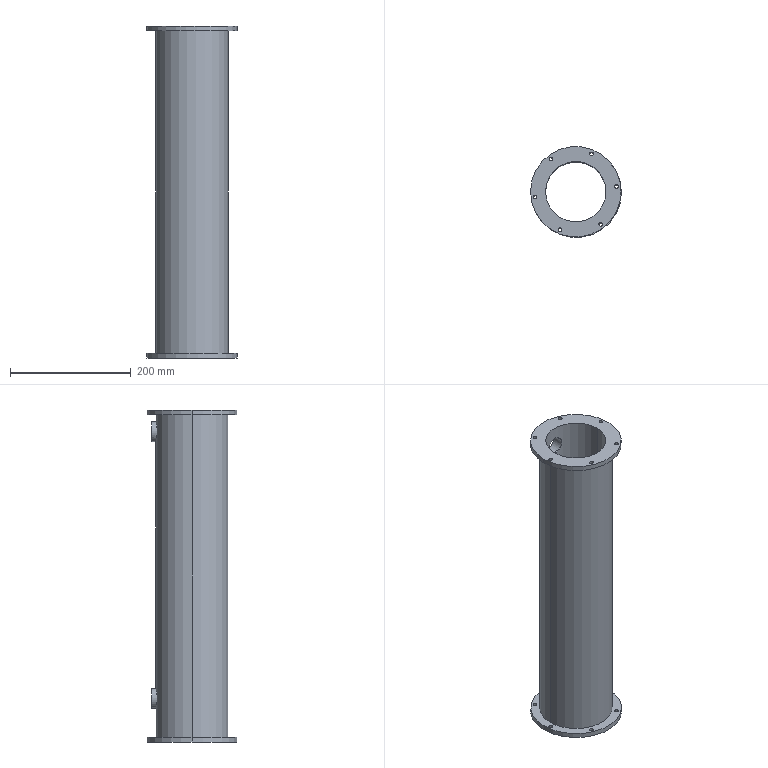Part | SolidWorks | features ICE 6, Chamfer 1, Extrusion 1 | 1 solid | 54 faces | box 150.705 x 150 x 550 mm | volume 1989302 mm3 | cylinder 40 | plane 6 | spline 4 | cone 4 | commonest cylinder face diameters 6 x24 29 x4 33 x4 150 x4 100 x2 120 x2